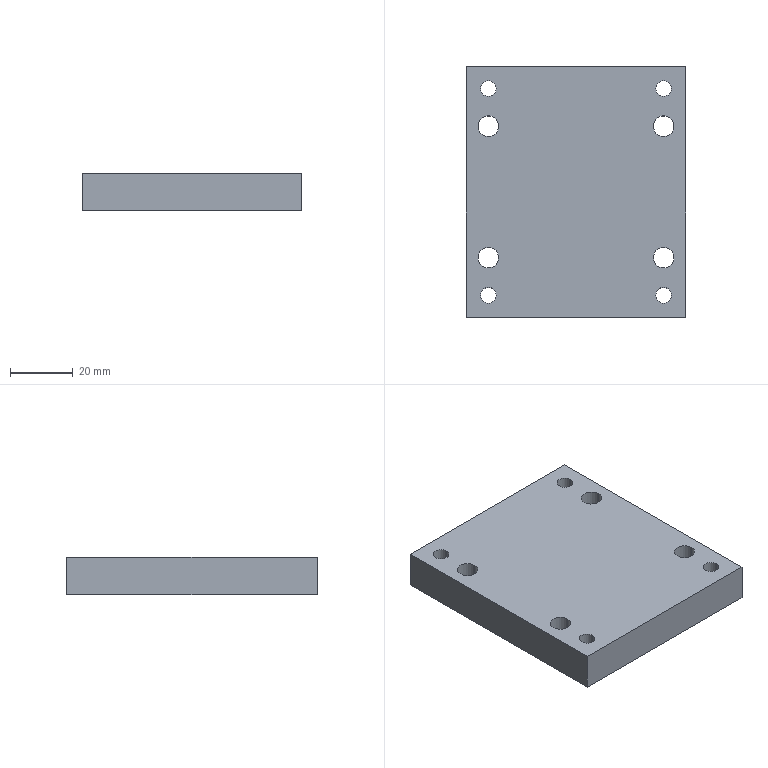Part | SolidWorks | features HoleWzd 2, Extrusion 1 | 1 solid | 34 faces | box 70 x 80 x 12 mm | volume 63058 mm3 | cylinder 24 | plane 10 | commonest cylinder face diameters 5 x8 6.6 x8 11 x8
STEP:
#1=CARTESIAN_POINT('',(33.5,-21.,6.4));
#2=VERTEX_POINT('',#1);
#3=CARTESIAN_POINT('',(22.5,-21.,6.4));
#4=VERTEX_POINT('',#3);
#5=CARTESIAN_POINT('',(28.,-21.,6.4));
#6=DIRECTION('',(0.,0.,-1.));
#7=DIRECTION('',(-1.,0.,0.));
#8=AXIS2_PLACEMENT_3D('',#5,#6,#7);
#9=CIRCLE('',#8,5.5);
#10=EDGE_CURVE('',#2,#4,#9,.T.);
#11=ORIENTED_EDGE('',*,*,#10,.F.);
#12=CARTESIAN_POINT('',(33.5,-21.,0.));
#13=VERTEX_POINT('',#12);
#14=CARTESIAN_POINT('',(33.5,-21.,0.));
#15=DIRECTION('',(0.,0.,-1.));
#16=VECTOR('',#15,1000.);
#17=LINE('',#14,#16);
#18=EDGE_CURVE('',#2,#13,#17,.T.);
#19=ORIENTED_EDGE('',*,*,#18,.T.);
#20=CARTESIAN_POINT('',(22.5,-21.,0.));
#21=VERTEX_POINT('',#20);
#22=CARTESIAN_POINT('',(28.,-21.,0.));
#23=DIRECTION('',(0.,0.,-1.));
#24=DIRECTION('',(-1.,0.,0.));
#25=AXIS2_PLACEMENT_3D('',#22,#23,#24);
#26=CIRCLE('',#25,5.5);
#27=EDGE_CURVE('',#13,#21,#26,.T.);
#28=ORIENTED_EDGE('',*,*,#27,.T.);
#29=CARTESIAN_POINT('',(22.5,-21.,0.));
#30=DIRECTION('',(0.,0.,-1.));
#31=VECTOR('',#30,1000.);
#32=LINE('',#29,#31);
#33=EDGE_CURVE('',#4,#21,#32,.T.);
#34=ORIENTED_EDGE('',*,*,#33,.F.);
#35=EDGE_LOOP('',(#11,#19,#28,#34));
#36=FACE_OUTER_BOUND('',#35,.T.);
#37=CARTESIAN_POINT('',(28.,-21.,0.));
#38=DIRECTION('',(0.,0.,-1.));
#39=DIRECTION('',(-1.,0.,0.));
#40=AXIS2_PLACEMENT_3D('',#37,#38,#39);
#41=CYLINDRICAL_SURFACE('',#40,5.5);
#42=ADVANCED_FACE('',(#36),#41,.F.);
#43=CARTESIAN_POINT('',(31.3,-21.,12.));
#44=VERTEX_POINT('',#43);
#45=CARTESIAN_POINT('',(24.7,-21.,12.));
#46=VERTEX_POINT('',#45);
#47=CARTESIAN_POINT('',(28.,-21.,12.));
#48=DIRECTION('',(0.,0.,-1.));
#49=DIRECTION('',(-1.,0.,0.));
#50=AXIS2_PLACEMENT_3D('',#47,#48,#49);
#51=CIRCLE('',#50,3.3);
#52=EDGE_CURVE('',#44,#46,#51,.T.);
#53=ORIENTED_EDGE('',*,*,#52,.F.);
#54=CARTESIAN_POINT('',(31.3,-21.,6.4));
#55=VERTEX_POINT('',#54);
#56=CARTESIAN_POINT('',(31.3,-21.,0.));
#57=DIRECTION('',(0.,0.,-1.));
#58=VECTOR('',#57,1000.);
#59=LINE('',#56,#58);
#60=EDGE_CURVE('',#44,#55,#59,.T.);
#61=ORIENTED_EDGE('',*,*,#60,.T.);
#62=CARTESIAN_POINT('',(24.7,-21.,6.4));
#63=VERTEX_POINT('',#62);
#64=CARTESIAN_POINT('',(28.,-21.,6.4));
#65=DIRECTION('',(0.,0.,-1.));
#66=DIRECTION('',(-1.,0.,0.));
#67=AXIS2_PLACEMENT_3D('',#64,#65,#66);
#68=CIRCLE('',#67,3.3);
#69=EDGE_CURVE('',#55,#63,#68,.T.);
#70=ORIENTED_EDGE('',*,*,#69,.T.);
#71=CARTESIAN_POINT('',(24.7,-21.,0.));
#72=DIRECTION('',(0.,0.,-1.));
#73=VECTOR('',#72,1000.);
#74=LINE('',#71,#73);
#75=EDGE_CURVE('',#46,#63,#74,.T.);
#76=ORIENTED_EDGE('',*,*,#75,.F.);
#77=EDGE_LOOP('',(#53,#61,#70,#76));
#78=FACE_OUTER_BOUND('',#77,.T.);
#79=CARTESIAN_POINT('',(28.,-21.,0.));
#80=DIRECTION('',(0.,0.,-1.));
#81=DIRECTION('',(-1.,0.,0.));
#82=AXIS2_PLACEMENT_3D('',#79,#80,#81);
#83=CYLINDRICAL_SURFACE('',#82,3.3);
#84=ADVANCED_FACE('',(#78),#83,.F.);
#85=CARTESIAN_POINT('',(33.5,21.,6.4));
#86=VERTEX_POINT('',#85);
#87=CARTESIAN_POINT('',(22.5,21.,6.4));
#88=VERTEX_POINT('',#87);
#89=CARTESIAN_POINT('',(28.,21.,6.4));
#90=DIRECTION('',(0.,0.,-1.));
#91=DIRECTION('',(-1.,0.,0.));
#92=AXIS2_PLACEMENT_3D('',#89,#90,#91);
#93=CIRCLE('',#92,5.5);
#94=EDGE_CURVE('',#86,#88,#93,.T.);
#95=ORIENTED_EDGE('',*,*,#94,.F.);
#96=CARTESIAN_POINT('',(33.5,21.,0.));
#97=VERTEX_POINT('',#96);
#98=CARTESIAN_POINT('',(33.5,21.,0.));
#99=DIRECTION('',(0.,0.,-1.));
#100=VECTOR('',#99,1000.);
#101=LINE('',#98,#100);
#102=EDGE_CURVE('',#86,#97,#101,.T.);
#103=ORIENTED_EDGE('',*,*,#102,.T.);
#104=CARTESIAN_POINT('',(22.5,21.,0.));
#105=VERTEX_POINT('',#104);
#106=CARTESIAN_POINT('',(28.,21.,0.));
#107=DIRECTION('',(0.,0.,-1.));
#108=DIRECTION('',(-1.,0.,0.));
#109=AXIS2_PLACEMENT_3D('',#106,#107,#108);
#110=CIRCLE('',#109,5.5);
#111=EDGE_CURVE('',#97,#105,#110,.T.);
#112=ORIENTED_EDGE('',*,*,#111,.T.);
#113=CARTESIAN_POINT('',(22.5,21.,0.));
#114=DIRECTION('',(0.,0.,-1.));
#115=VECTOR('',#114,1000.);
#116=LINE('',#113,#115);
#117=EDGE_CURVE('',#88,#105,#116,.T.);
#118=ORIENTED_EDGE('',*,*,#117,.F.);
#119=EDGE_LOOP('',(#95,#103,#112,#118));
#120=FACE_OUTER_BOUND('',#119,.T.);
#121=CARTESIAN_POINT('',(28.,21.,0.));
#122=DIRECTION('',(0.,0.,-1.));
#123=DIRECTION('',(-1.,0.,0.));
#124=AXIS2_PLACEMENT_3D('',#121,#122,#123);
#125=CYLINDRICAL_SURFACE('',#124,5.5);
#126=ADVANCED_FACE('',(#120),#125,.F.);
#127=CARTESIAN_POINT('',(31.3,21.,12.));
#128=VERTEX_POINT('',#127);
#129=CARTESIAN_POINT('',(24.7,21.,12.));
#130=VERTEX_POINT('',#129);
#131=CARTESIAN_POINT('',(28.,21.,12.));
#132=DIRECTION('',(0.,0.,-1.));
#133=DIRECTION('',(-1.,0.,0.));
#134=AXIS2_PLACEMENT_3D('',#131,#132,#133);
#135=CIRCLE('',#134,3.3);
#136=EDGE_CURVE('',#128,#130,#135,.T.);
#137=ORIENTED_EDGE('',*,*,#136,.F.);
#138=CARTESIAN_POINT('',(31.3,21.,6.4));
#139=VERTEX_POINT('',#138);
#140=CARTESIAN_POINT('',(31.3,21.,0.));
#141=DIRECTION('',(0.,0.,-1.));
#142=VECTOR('',#141,1000.);
#143=LINE('',#140,#142);
#144=EDGE_CURVE('',#128,#139,#143,.T.);
#145=ORIENTED_EDGE('',*,*,#144,.T.);
#146=CARTESIAN_POINT('',(24.7,21.,6.4));
#147=VERTEX_POINT('',#146);
#148=CARTESIAN_POINT('',(28.,21.,6.4));
#149=DIRECTION('',(0.,0.,-1.));
#150=DIRECTION('',(-1.,0.,0.));
#151=AXIS2_PLACEMENT_3D('',#148,#149,#150);
#152=CIRCLE('',#151,3.3);
#153=EDGE_CURVE('',#139,#147,#152,.T.);
#154=ORIENTED_EDGE('',*,*,#153,.T.);
#155=CARTESIAN_POINT('',(24.7,21.,0.));
#156=DIRECTION('',(0.,0.,-1.));
#157=VECTOR('',#156,1000.);
#158=LINE('',#155,#157);
#159=EDGE_CURVE('',#130,#147,#158,.T.);
#160=ORIENTED_EDGE('',*,*,#159,.F.);
#161=EDGE_LOOP('',(#137,#145,#154,#160));
#162=FACE_OUTER_BOUND('',#161,.T.);
#163=CARTESIAN_POINT('',(28.,21.,0.));
#164=DIRECTION('',(0.,0.,-1.));
#165=DIRECTION('',(-1.,0.,0.));
#166=AXIS2_PLACEMENT_3D('',#163,#164,#165);
#167=CYLINDRICAL_SURFACE('',#166,3.3);
#168=ADVANCED_FACE('',(#162),#167,.F.);
#169=CARTESIAN_POINT('',(-22.5,-21.,6.4));
#170=VERTEX_POINT('',#169);
#171=CARTESIAN_POINT('',(-33.5,-21.,6.4));
#172=VERTEX_POINT('',#171);
#173=CARTESIAN_POINT('',(-28.,-21.,6.4));
#174=DIRECTION('',(0.,0.,-1.));
#175=DIRECTION('',(-1.,0.,0.));
#176=AXIS2_PLACEMENT_3D('',#173,#174,#175);
#177=CIRCLE('',#176,5.5);
#178=EDGE_CURVE('',#170,#172,#177,.T.);
#179=ORIENTED_EDGE('',*,*,#178,.F.);
#180=CARTESIAN_POINT('',(-22.5,-21.,0.));
#181=VERTEX_POINT('',#180);
#182=CARTESIAN_POINT('',(-22.5,-21.,0.));
#183=DIRECTION('',(0.,0.,-1.));
#184=VECTOR('',#183,1000.);
#185=LINE('',#182,#184);
#186=EDGE_CURVE('',#170,#181,#185,.T.);
#187=ORIENTED_EDGE('',*,*,#186,.T.);
#188=CARTESIAN_POINT('',(-33.5,-21.,0.));
#189=VERTEX_POINT('',#188);
#190=CARTESIAN_POINT('',(-28.,-21.,0.));
#191=DIRECTION('',(0.,0.,-1.));
#192=DIRECTION('',(-1.,0.,0.));
#193=AXIS2_PLACEMENT_3D('',#190,#191,#192);
#194=CIRCLE('',#193,5.5);
#195=EDGE_CURVE('',#181,#189,#194,.T.);
#196=ORIENTED_EDGE('',*,*,#195,.T.);
#197=CARTESIAN_POINT('',(-33.5,-21.,0.));
#198=DIRECTION('',(0.,0.,-1.));
#199=VECTOR('',#198,1000.);
#200=LINE('',#197,#199);
#201=EDGE_CURVE('',#172,#189,#200,.T.);
#202=ORIENTED_EDGE('',*,*,#201,.F.);
#203=EDGE_LOOP('',(#179,#187,#196,#202));
#204=FACE_OUTER_BOUND('',#203,.T.);
#205=CARTESIAN_POINT('',(-28.,-21.,0.));
#206=DIRECTION('',(0.,0.,-1.));
#207=DIRECTION('',(-1.,0.,0.));
#208=AXIS2_PLACEMENT_3D('',#205,#206,#207);
#209=CYLINDRICAL_SURFACE('',#208,5.5);
#210=ADVANCED_FACE('',(#204),#209,.F.);
#211=CARTESIAN_POINT('',(-24.7,-21.,12.));
#212=VERTEX_POINT('',#211);
#213=CARTESIAN_POINT('',(-31.3,-21.,12.));
#214=VERTEX_POINT('',#213);
#215=CARTESIAN_POINT('',(-28.,-21.,12.));
#216=DIRECTION('',(0.,0.,-1.));
#217=DIRECTION('',(-1.,0.,0.));
#218=AXIS2_PLACEMENT_3D('',#215,#216,#217);
#219=CIRCLE('',#218,3.3);
#220=EDGE_CURVE('',#212,#214,#219,.T.);
#221=ORIENTED_EDGE('',*,*,#220,.F.);
#222=CARTESIAN_POINT('',(-24.7,-21.,6.4));
#223=VERTEX_POINT('',#222);
#224=CARTESIAN_POINT('',(-24.7,-21.,0.));
#225=DIRECTION('',(0.,0.,-1.));
#226=VECTOR('',#225,1000.);
#227=LINE('',#224,#226);
#228=EDGE_CURVE('',#212,#223,#227,.T.);
#229=ORIENTED_EDGE('',*,*,#228,.T.);
#230=CARTESIAN_POINT('',(-31.3,-21.,6.4));
#231=VERTEX_POINT('',#230);
#232=CARTESIAN_POINT('',(-28.,-21.,6.4));
#233=DIRECTION('',(0.,0.,-1.));
#234=DIRECTION('',(-1.,0.,0.));
#235=AXIS2_PLACEMENT_3D('',#232,#233,#234);
#236=CIRCLE('',#235,3.3);
#237=EDGE_CURVE('',#223,#231,#236,.T.);
#238=ORIENTED_EDGE('',*,*,#237,.T.);
#239=CARTESIAN_POINT('',(-31.3,-21.,0.));
#240=DIRECTION('',(0.,0.,-1.));
#241=VECTOR('',#240,1000.);
#242=LINE('',#239,#241);
#243=EDGE_CURVE('',#214,#231,#242,.T.);
#244=ORIENTED_EDGE('',*,*,#243,.F.);
#245=EDGE_LOOP('',(#221,#229,#238,#244));
#246=FACE_OUTER_BOUND('',#245,.T.);
#247=CARTESIAN_POINT('',(-28.,-21.,0.));
#248=DIRECTION('',(0.,0.,-1.));
#249=DIRECTION('',(-1.,0.,0.));
#250=AXIS2_PLACEMENT_3D('',#247,#248,#249);
#251=CYLINDRICAL_SURFACE('',#250,3.3);
#252=ADVANCED_FACE('',(#246),#251,.F.);
#253=CARTESIAN_POINT('',(-22.5,21.,6.4));
#254=VERTEX_POINT('',#253);
#255=CARTESIAN_POINT('',(-33.5,21.,6.4));
#256=VERTEX_POINT('',#255);
#257=CARTESIAN_POINT('',(-28.,21.,6.4));
#258=DIRECTION('',(0.,0.,-1.));
#259=DIRECTION('',(-1.,0.,0.));
#260=AXIS2_PLACEMENT_3D('',#257,#258,#259);
#261=CIRCLE('',#260,5.5);
#262=EDGE_CURVE('',#254,#256,#261,.T.);
#263=ORIENTED_EDGE('',*,*,#262,.F.);
#264=CARTESIAN_POINT('',(-22.5,21.,0.));
#265=VERTEX_POINT('',#264);
#266=CARTESIAN_POINT('',(-22.5,21.,0.));
#267=DIRECTION('',(0.,0.,-1.));
#268=VECTOR('',#267,1000.);
#269=LINE('',#266,#268);
#270=EDGE_CURVE('',#254,#265,#269,.T.);
#271=ORIENTED_EDGE('',*,*,#270,.T.);
#272=CARTESIAN_POINT('',(-33.5,21.,0.));
#273=VERTEX_POINT('',#272);
#274=CARTESIAN_POINT('',(-28.,21.,0.));
#275=DIRECTION('',(0.,0.,-1.));
#276=DIRECTION('',(-1.,0.,0.));
#277=AXIS2_PLACEMENT_3D('',#274,#275,#276);
#278=CIRCLE('',#277,5.5);
#279=EDGE_CURVE('',#265,#273,#278,.T.);
#280=ORIENTED_EDGE('',*,*,#279,.T.);
#281=CARTESIAN_POINT('',(-33.5,21.,0.));
#282=DIRECTION('',(0.,0.,-1.));
#283=VECTOR('',#282,1000.);
#284=LINE('',#281,#283);
#285=EDGE_CURVE('',#256,#273,#284,.T.);
#286=ORIENTED_EDGE('',*,*,#285,.F.);
#287=EDGE_LOOP('',(#263,#271,#280,#286));
#288=FACE_OUTER_BOUND('',#287,.T.);
#289=CARTESIAN_POINT('',(-28.,21.,0.));
#290=DIRECTION('',(0.,0.,-1.));
#291=DIRECTION('',(-1.,0.,0.));
#292=AXIS2_PLACEMENT_3D('',#289,#290,#291);
#293=CYLINDRICAL_SURFACE('',#292,5.5);
#294=ADVANCED_FACE('',(#288),#293,.F.);
#295=CARTESIAN_POINT('',(-24.7,21.,12.));
#296=VERTEX_POINT('',#295);
#297=CARTESIAN_POINT('',(-31.3,21.,12.));
#298=VERTEX_POINT('',#297);
#299=CARTESIAN_POINT('',(-28.,21.,12.));
#300=DIRECTION('',(0.,0.,-1.));
#301=DIRECTION('',(-1.,0.,0.));
#302=AXIS2_PLACEMENT_3D('',#299,#300,#301);
#303=CIRCLE('',#302,3.3);
#304=EDGE_CURVE('',#296,#298,#303,.T.);
#305=ORIENTED_EDGE('',*,*,#304,.F.);
#306=CARTESIAN_POINT('',(-24.7,21.,6.4));
#307=VERTEX_POINT('',#306);
#308=CARTESIAN_POINT('',(-24.7,21.,0.));
#309=DIRECTION('',(0.,0.,-1.));
#310=VECTOR('',#309,1000.);
#311=LINE('',#308,#310);
#312=EDGE_CURVE('',#296,#307,#311,.T.);
#313=ORIENTED_EDGE('',*,*,#312,.T.);
#314=CARTESIAN_POINT('',(-31.3,21.,6.4));
#315=VERTEX_POINT('',#314);
#316=CARTESIAN_POINT('',(-28.,21.,6.4));
#317=DIRECTION('',(0.,0.,-1.));
#318=DIRECTION('',(-1.,0.,0.));
#319=AXIS2_PLACEMENT_3D('',#316,#317,#318);
#320=CIRCLE('',#319,3.3);
#321=EDGE_CURVE('',#307,#315,#320,.T.);
#322=ORIENTED_EDGE('',*,*,#321,.T.);
#323=CARTESIAN_POINT('',(-31.3,21.,0.));
#324=DIRECTION('',(0.,0.,-1.));
#325=VECTOR('',#324,1000.);
#326=LINE('',#323,#325);
#327=EDGE_CURVE('',#298,#315,#326,.T.);
#328=ORIENTED_EDGE('',*,*,#327,.F.);
#329=EDGE_LOOP('',(#305,#313,#322,#328));
#330=FACE_OUTER_BOUND('',#329,.T.);
#331=CARTESIAN_POINT('',(-28.,21.,0.));
#332=DIRECTION('',(0.,0.,-1.));
#333=DIRECTION('',(-1.,0.,0.));
#334=AXIS2_PLACEMENT_3D('',#331,#332,#333);
#335=CYLINDRICAL_SURFACE('',#334,3.3);
#336=ADVANCED_FACE('',(#330),#335,.F.);
#337=CARTESIAN_POINT('',(-25.5,33.,12.));
#338=VERTEX_POINT('',#337);
#339=CARTESIAN_POINT('',(-30.5,33.,12.));
#340=VERTEX_POINT('',#339);
#341=CARTESIAN_POINT('',(-28.,33.,12.));
#342=DIRECTION('',(0.,0.,-1.));
#343=DIRECTION('',(-1.,0.,0.));
#344=AXIS2_PLACEMENT_3D('',#341,#342,#343);
#345=CIRCLE('',#344,2.5);
#346=EDGE_CURVE('',#338,#340,#345,.T.);
#347=ORIENTED_EDGE('',*,*,#346,.F.);
#348=CARTESIAN_POINT('',(-25.5,33.,0.));
#349=VERTEX_POINT('',#348);
#350=CARTESIAN_POINT('',(-25.5,33.,0.));
#351=DIRECTION('',(0.,0.,-1.));
#352=VECTOR('',#351,1000.);
#353=LINE('',#350,#352);
#354=EDGE_CURVE('',#338,#349,#353,.T.);
#355=ORIENTED_EDGE('',*,*,#354,.T.);
#356=CARTESIAN_POINT('',(-30.5,33.,0.));
#357=VERTEX_POINT('',#356);
#358=CARTESIAN_POINT('',(-28.,33.,0.));
#359=DIRECTION('',(0.,0.,-1.));
#360=DIRECTION('',(-1.,0.,0.));
#361=AXIS2_PLACEMENT_3D('',#358,#359,#360);
#362=CIRCLE('',#361,2.5);
#363=EDGE_CURVE('',#349,#357,#362,.T.);
#364=ORIENTED_EDGE('',*,*,#363,.T.);
#365=CARTESIAN_POINT('',(-30.5,33.,0.));
#366=DIRECTION('',(0.,0.,-1.));
#367=VECTOR('',#366,1000.);
#368=LINE('',#365,#367);
#369=EDGE_CURVE('',#340,#357,#368,.T.);
#370=ORIENTED_EDGE('',*,*,#369,.F.);
#371=EDGE_LOOP('',(#347,#355,#364,#370));
#372=FACE_OUTER_BOUND('',#371,.T.);
#373=CARTESIAN_POINT('',(-28.,33.,0.));
#374=DIRECTION('',(0.,0.,-1.));
#375=DIRECTION('',(-1.,0.,0.));
#376=AXIS2_PLACEMENT_3D('',#373,#374,#375);
#377=CYLINDRICAL_SURFACE('',#376,2.5);
#378=ADVANCED_FACE('',(#372),#377,.F.);
#379=CARTESIAN_POINT('',(-25.5,-33.,12.));
#380=VERTEX_POINT('',#379);
#381=CARTESIAN_POINT('',(-30.5,-33.,12.));
#382=VERTEX_POINT('',#381);
#383=CARTESIAN_POINT('',(-28.,-33.,12.));
#384=DIRECTION('',(0.,0.,-1.));
#385=DIRECTION('',(-1.,0.,0.));
#386=AXIS2_PLACEMENT_3D('',#383,#384,#385);
#387=CIRCLE('',#386,2.5);
#388=EDGE_CURVE('',#380,#382,#387,.T.);
#389=ORIENTED_EDGE('',*,*,#388,.F.);
#390=CARTESIAN_POINT('',(-25.5,-33.,0.));
#391=VERTEX_POINT('',#390);
#392=CARTESIAN_POINT('',(-25.5,-33.,0.));
#393=DIRECTION('',(0.,0.,-1.));
#394=VECTOR('',#393,1000.);
#395=LINE('',#392,#394);
#396=EDGE_CURVE('',#380,#391,#395,.T.);
#397=ORIENTED_EDGE('',*,*,#396,.T.);
#398=CARTESIAN_POINT('',(-30.5,-33.,0.));
#399=VERTEX_POINT('',#398);
#400=CARTESIAN_POINT('',(-28.,-33.,0.));
#401=DIRECTION('',(0.,0.,-1.));
#402=DIRECTION('',(-1.,0.,0.));
#403=AXIS2_PLACEMENT_3D('',#400,#401,#402);
#404=CIRCLE('',#403,2.5);
#405=EDGE_CURVE('',#391,#399,#404,.T.);
#406=ORIENTED_EDGE('',*,*,#405,.T.);
#407=CARTESIAN_POINT('',(-30.5,-33.,0.));
#408=DIRECTION('',(0.,0.,-1.));
#409=VECTOR('',#408,1000.);
#410=LINE('',#407,#409);
#411=EDGE_CURVE('',#382,#399,#410,.T.);
#412=ORIENTED_EDGE('',*,*,#411,.F.);
#413=EDGE_LOOP('',(#389,#397,#406,#412));
#414=FACE_OUTER_BOUND('',#413,.T.);
#415=CARTESIAN_POINT('',(-28.,-33.,0.));
#416=DIRECTION('',(0.,0.,-1.));
#417=DIRECTION('',(-1.,0.,0.));
#418=AXIS2_PLACEMENT_3D('',#415,#416,#417);
#419=CYLINDRICAL_SURFACE('',#418,2.5);
#420=ADVANCED_FACE('',(#414),#419,.F.);
#421=CARTESIAN_POINT('',(30.5,-33.,12.));
#422=VERTEX_POINT('',#421);
#423=CARTESIAN_POINT('',(25.5,-33.,12.));
#424=VERTEX_POINT('',#423);
#425=CARTESIAN_POINT('',(28.,-33.,12.));
#426=DIRECTION('',(0.,0.,-1.));
#427=DIRECTION('',(-1.,0.,0.));
#428=AXIS2_PLACEMENT_3D('',#425,#426,#427);
#429=CIRCLE('',#428,2.5);
#430=EDGE_CURVE('',#422,#424,#429,.T.);
#431=ORIENTED_EDGE('',*,*,#430,.F.);
#432=CARTESIAN_POINT('',(30.5,-33.,0.));
#433=VERTEX_POINT('',#432);
#434=CARTESIAN_POINT('',(30.5,-33.,0.));
#435=DIRECTION('',(0.,0.,-1.));
#436=VECTOR('',#435,1000.);
#437=LINE('',#434,#436);
#438=EDGE_CURVE('',#422,#433,#437,.T.);
#439=ORIENTED_EDGE('',*,*,#438,.T.);
#440=CARTESIAN_POINT('',(25.5,-33.,0.));
#441=VERTEX_POINT('',#440);
#442=CARTESIAN_POINT('',(28.,-33.,0.));
#443=DIRECTION('',(0.,0.,-1.));
#444=DIRECTION('',(-1.,0.,0.));
#445=AXIS2_PLACEMENT_3D('',#442,#443,#444);
#446=CIRCLE('',#445,2.5);
#447=EDGE_CURVE('',#433,#441,#446,.T.);
#448=ORIENTED_EDGE('',*,*,#447,.T.);
#449=CARTESIAN_POINT('',(25.5,-33.,0.));
#450=DIRECTION('',(0.,0.,-1.));
#451=VECTOR('',#450,1000.);
#452=LINE('',#449,#451);
#453=EDGE_CURVE('',#424,#441,#452,.T.);
#454=ORIENTED_EDGE('',*,*,#453,.F.);
#455=EDGE_LOOP('',(#431,#439,#448,#454));
#456=FACE_OUTER_BOUND('',#455,.T.);
#457=CARTESIAN_POINT('',(28.,-33.,0.));
#458=DIRECTION('',(0.,0.,-1.));
#459=DIRECTION('',(-1.,0.,0.));
#460=AXIS2_PLACEMENT_3D('',#457,#458,#459);
#461=CYLINDRICAL_SURFACE('',#460,2.5);
#462=ADVANCED_FACE('',(#456),#461,.F.);
#463=CARTESIAN_POINT('',(30.5,33.,12.));
#464=VERTEX_POINT('',#463);
#465=CARTESIAN_POINT('',(25.5,33.,12.));
#466=VERTEX_POINT('',#465);
#467=CARTESIAN_POINT('',(28.,33.,12.));
#468=DIRECTION('',(0.,0.,-1.));
#469=DIRECTION('',(-1.,0.,0.));
#470=AXIS2_PLACEMENT_3D('',#467,#468,#469);
#471=CIRCLE('',#470,2.5);
#472=EDGE_CURVE('',#464,#466,#471,.T.);
#473=ORIENTED_EDGE('',*,*,#472,.F.);
#474=CARTESIAN_POINT('',(30.5,33.,0.));
#475=VERTEX_POINT('',#474);
#476=CARTESIAN_POINT('',(30.5,33.,0.));
#477=DIRECTION('',(0.,0.,-1.));
#478=VECTOR('',#477,1000.);
#479=LINE('',#476,#478);
#480=EDGE_CURVE('',#464,#475,#479,.T.);
#481=ORIENTED_EDGE('',*,*,#480,.T.);
#482=CARTESIAN_POINT('',(25.5,33.,0.));
#483=VERTEX_POINT('',#482);
#484=CARTESIAN_POINT('',(28.,33.,0.));
#485=DIRECTION('',(0.,0.,-1.));
#486=DIRECTION('',(-1.,0.,0.));
#487=AXIS2_PLACEMENT_3D('',#484,#485,#486);
#488=CIRCLE('',#487,2.5);
#489=EDGE_CURVE('',#475,#483,#488,.T.);
#490=ORIENTED_EDGE('',*,*,#489,.T.);
#491=CARTESIAN_POINT('',(25.5,33.,0.));
#492=DIRECTION('',(0.,0.,-1.));
#493=VECTOR('',#492,1000.);
#494=LINE('',#491,#493);
#495=EDGE_CURVE('',#466,#483,#494,.T.);
#496=ORIENTED_EDGE('',*,*,#495,.F.);
#497=EDGE_LOOP('',(#473,#481,#490,#496));
#498=FACE_OUTER_BOUND('',#497,.T.);
#499=CARTESIAN_POINT('',(28.,33.,0.));
#500=DIRECTION('',(0.,0.,-1.));
#501=DIRECTION('',(-1.,0.,0.));
#502=AXIS2_PLACEMENT_3D('',#499,#500,#501);
#503=CYLINDRICAL_SURFACE('',#502,2.5);
#504=ADVANCED_FACE('',(#498),#503,.F.);
#505=CARTESIAN_POINT('',(35.,-40.,0.));
#506=VERTEX_POINT('',#505);
#507=CARTESIAN_POINT('',(35.,40.,0.));
#508=VERTEX_POINT('',#507);
#509=CARTESIAN_POINT('',(35.,40.,0.));
#510=DIRECTION('',(0.,1.,0.));
#511=VECTOR('',#510,1000.);
#512=LINE('',#509,#511);
#513=EDGE_CURVE('',#506,#508,#512,.T.);
#514=ORIENTED_EDGE('',*,*,#513,.T.);
#515=CARTESIAN_POINT('',(35.,40.,12.));
#516=VERTEX_POINT('',#515);
#517=CARTESIAN_POINT('',(35.,40.,12.));
#518=DIRECTION('',(0.,0.,-1.));
#519=VECTOR('',#518,1000.);
#520=LINE('',#517,#519);
#521=EDGE_CURVE('',#516,#508,#520,.T.);
#522=ORIENTED_EDGE('',*,*,#521,.F.);
#523=CARTESIAN_POINT('',(35.,-40.,12.));
#524=VERTEX_POINT('',#523);
#525=CARTESIAN_POINT('',(35.,40.,12.));
#526=DIRECTION('',(0.,1.,0.));
#527=VECTOR('',#526,1000.);
#528=LINE('',#525,#527);
#529=EDGE_CURVE('',#524,#516,#528,.T.);
#530=ORIENTED_EDGE('',*,*,#529,.F.);
#531=CARTESIAN_POINT('',(35.,-40.,12.));
#532=DIRECTION('',(0.,0.,-1.));
#533=VECTOR('',#532,1000.);
#534=LINE('',#531,#533);
#535=EDGE_CURVE('',#524,#506,#534,.T.);
#536=ORIENTED_EDGE('',*,*,#535,.T.);
#537=EDGE_LOOP('',(#514,#522,#530,#536));
#538=FACE_OUTER_BOUND('',#537,.T.);
#539=CARTESIAN_POINT('',(35.,40.,12.));
#540=DIRECTION('',(-1.,0.,0.));
#541=DIRECTION('',(0.,-1.,0.));
#542=AXIS2_PLACEMENT_3D('',#539,#540,#541);
#543=PLANE('',#542);
#544=ADVANCED_FACE('',(#538),#543,.F.);
#545=CARTESIAN_POINT('',(-35.,40.,0.));
#546=VERTEX_POINT('',#545);
#547=CARTESIAN_POINT('',(-35.,40.,0.));
#548=DIRECTION('',(-1.,0.,0.));
#549=VECTOR('',#548,1000.);
#550=LINE('',#547,#549);
#551=EDGE_CURVE('',#508,#546,#550,.T.);
#552=ORIENTED_EDGE('',*,*,#551,.T.);
#553=CARTESIAN_POINT('',(-35.,40.,12.));
#554=VERTEX_POINT('',#553);
#555=CARTESIAN_POINT('',(-35.,40.,12.));
#556=DIRECTION('',(0.,0.,-1.));
#557=VECTOR('',#556,1000.);
#558=LINE('',#555,#557);
#559=EDGE_CURVE('',#554,#546,#558,.T.);
#560=ORIENTED_EDGE('',*,*,#559,.F.);
#561=CARTESIAN_POINT('',(-35.,40.,12.));
#562=DIRECTION('',(-1.,0.,0.));
#563=VECTOR('',#562,1000.);
#564=LINE('',#561,#563);
#565=EDGE_CURVE('',#516,#554,#564,.T.);
#566=ORIENTED_EDGE('',*,*,#565,.F.);
#567=ORIENTED_EDGE('',*,*,#521,.T.);
#568=EDGE_LOOP('',(#552,#560,#566,#567));
#569=FACE_OUTER_BOUND('',#568,.T.);
#570=CARTESIAN_POINT('',(-35.,40.,12.));
#571=DIRECTION('',(0.,-1.,0.));
#572=DIRECTION('',(0.,0.,-1.));
#573=AXIS2_PLACEMENT_3D('',#570,#571,#572);
#574=PLANE('',#573);
#575=ADVANCED_FACE('',(#569),#574,.F.);
#576=CARTESIAN_POINT('',(-35.,-40.,0.));
#577=VERTEX_POINT('',#576);
#578=CARTESIAN_POINT('',(-35.,40.,0.));
#579=DIRECTION('',(0.,-1.,0.));
#580=VECTOR('',#579,1000.);
#581=LINE('',#578,#580);
#582=EDGE_CURVE('',#546,#577,#581,.T.);
#583=ORIENTED_EDGE('',*,*,#582,.T.);
#584=CARTESIAN_POINT('',(-35.,-40.,12.));
#585=VERTEX_POINT('',#584);
#586=CARTESIAN_POINT('',(-35.,-40.,12.));
#587=DIRECTION('',(0.,0.,-1.));
#588=VECTOR('',#587,1000.);
#589=LINE('',#586,#588);
#590=EDGE_CURVE('',#585,#577,#589,.T.);
#591=ORIENTED_EDGE('',*,*,#590,.F.);
#592=CARTESIAN_POINT('',(-35.,40.,12.));
#593=DIRECTION('',(0.,-1.,0.));
#594=VECTOR('',#593,1000.);
#595=LINE('',#592,#594);
#596=EDGE_CURVE('',#554,#585,#595,.T.);
#597=ORIENTED_EDGE('',*,*,#596,.F.);
#598=ORIENTED_EDGE('',*,*,#559,.T.);
#599=EDGE_LOOP('',(#583,#591,#597,#598));
#600=FACE_OUTER_BOUND('',#599,.T.);
#601=CARTESIAN_POINT('',(-35.,40.,12.));
#602=DIRECTION('',(1.,0.,0.));
#603=DIRECTION('',(0.,0.,-1.));
#604=AXIS2_PLACEMENT_3D('',#601,#602,#603);
#605=PLANE('',#604);
#606=ADVANCED_FACE('',(#600),#605,.F.);
#607=CARTESIAN_POINT('',(-35.,-40.,0.));
#608=DIRECTION('',(1.,0.,0.));
#609=VECTOR('',#608,1000.);
#610=LINE('',#607,#609);
#611=EDGE_CURVE('',#577,#506,#610,.T.);
#612=ORIENTED_EDGE('',*,*,#611,.T.);
#613=ORIENTED_EDGE('',*,*,#535,.F.);
#614=CARTESIAN_POINT('',(-35.,-40.,12.));
#615=DIRECTION('',(1.,0.,0.));
#616=VECTOR('',#615,1000.);
#617=LINE('',#614,#616);
#618=EDGE_CURVE('',#585,#524,#617,.T.);
#619=ORIENTED_EDGE('',*,*,#618,.F.);
#620=ORIENTED_EDGE('',*,*,#590,.T.);
#621=EDGE_LOOP('',(#612,#613,#619,#620));
#622=FACE_OUTER_BOUND('',#621,.T.);
#623=CARTESIAN_POINT('',(-35.,-40.,12.));
#624=DIRECTION('',(0.,1.,0.));
#625=DIRECTION('',(0.,0.,1.));
#626=AXIS2_PLACEMENT_3D('',#623,#624,#625);
#627=PLANE('',#626);
#628=ADVANCED_FACE('',(#622),#627,.F.);
#629=CARTESIAN_POINT('',(28.,-21.,12.));
#630=DIRECTION('',(0.,0.,-1.));
#631=DIRECTION('',(-1.,0.,0.));
#632=AXIS2_PLACEMENT_3D('',#629,#630,#631);
#633=CIRCLE('',#632,3.3);
#634=EDGE_CURVE('',#46,#44,#633,.T.);
#635=ORIENTED_EDGE('',*,*,#634,.T.);
#636=ORIENTED_EDGE('',*,*,#52,.T.);
#637=EDGE_LOOP('',(#635,#636));
#638=FACE_BOUND('',#637,.T.);
#639=CARTESIAN_POINT('',(28.,21.,12.));
#640=DIRECTION('',(0.,0.,-1.));
#641=DIRECTION('',(-1.,0.,0.));
#642=AXIS2_PLACEMENT_3D('',#639,#640,#641);
#643=CIRCLE('',#642,3.3);
#644=EDGE_CURVE('',#130,#128,#643,.T.);
#645=ORIENTED_EDGE('',*,*,#644,.T.);
#646=ORIENTED_EDGE('',*,*,#136,.T.);
#647=EDGE_LOOP('',(#645,#646));
#648=FACE_BOUND('',#647,.T.);
#649=CARTESIAN_POINT('',(-28.,-21.,12.));
#650=DIRECTION('',(0.,0.,-1.));
#651=DIRECTION('',(-1.,0.,0.));
#652=AXIS2_PLACEMENT_3D('',#649,#650,#651);
#653=CIRCLE('',#652,3.3);
#654=EDGE_CURVE('',#214,#212,#653,.T.);
#655=ORIENTED_EDGE('',*,*,#654,.T.);
#656=ORIENTED_EDGE('',*,*,#220,.T.);
#657=EDGE_LOOP('',(#655,#656));
#658=FACE_BOUND('',#657,.T.);
#659=CARTESIAN_POINT('',(-28.,21.,12.));
#660=DIRECTION('',(0.,0.,-1.));
#661=DIRECTION('',(-1.,0.,0.));
#662=AXIS2_PLACEMENT_3D('',#659,#660,#661);
#663=CIRCLE('',#662,3.3);
#664=EDGE_CURVE('',#298,#296,#663,.T.);
#665=ORIENTED_EDGE('',*,*,#664,.T.);
#666=ORIENTED_EDGE('',*,*,#304,.T.);
#667=EDGE_LOOP('',(#665,#666));
#668=FACE_BOUND('',#667,.T.);
#669=CARTESIAN_POINT('',(-28.,33.,12.));
#670=DIRECTION('',(0.,0.,-1.));
#671=DIRECTION('',(-1.,0.,0.));
#672=AXIS2_PLACEMENT_3D('',#669,#670,#671);
#673=CIRCLE('',#672,2.5);
#674=EDGE_CURVE('',#340,#338,#673,.T.);
#675=ORIENTED_EDGE('',*,*,#674,.T.);
#676=ORIENTED_EDGE('',*,*,#346,.T.);
#677=EDGE_LOOP('',(#675,#676));
#678=FACE_BOUND('',#677,.T.);
#679=CARTESIAN_POINT('',(-28.,-33.,12.));
#680=DIRECTION('',(0.,0.,-1.));
#681=DIRECTION('',(-1.,0.,0.));
#682=AXIS2_PLACEMENT_3D('',#679,#680,#681);
#683=CIRCLE('',#682,2.5);
#684=EDGE_CURVE('',#382,#380,#683,.T.);
#685=ORIENTED_EDGE('',*,*,#684,.T.);
#686=ORIENTED_EDGE('',*,*,#388,.T.);
#687=EDGE_LOOP('',(#685,#686));
#688=FACE_BOUND('',#687,.T.);
#689=CARTESIAN_POINT('',(28.,-33.,12.));
#690=DIRECTION('',(0.,0.,-1.));
#691=DIRECTION('',(-1.,0.,0.));
#692=AXIS2_PLACEMENT_3D('',#689,#690,#691);
#693=CIRCLE('',#692,2.5);
#694=EDGE_CURVE('',#424,#422,#693,.T.);
#695=ORIENTED_EDGE('',*,*,#694,.T.);
#696=ORIENTED_EDGE('',*,*,#430,.T.);
#697=EDGE_LOOP('',(#695,#696));
#698=FACE_BOUND('',#697,.T.);
#699=CARTESIAN_POINT('',(28.,33.,12.));
#700=DIRECTION('',(0.,0.,-1.));
#701=DIRECTION('',(-1.,0.,0.));
#702=AXIS2_PLACEMENT_3D('',#699,#700,#701);
#703=CIRCLE('',#702,2.5);
#704=EDGE_CURVE('',#466,#464,#703,.T.);
#705=ORIENTED_EDGE('',*,*,#704,.T.);
#706=ORIENTED_EDGE('',*,*,#472,.T.);
#707=EDGE_LOOP('',(#705,#706));
#708=FACE_BOUND('',#707,.T.);
#709=ORIENTED_EDGE('',*,*,#529,.T.);
#710=ORIENTED_EDGE('',*,*,#565,.T.);
#711=ORIENTED_EDGE('',*,*,#596,.T.);
#712=ORIENTED_EDGE('',*,*,#618,.T.);
#713=EDGE_LOOP('',(#709,#710,#711,#712));
#714=FACE_OUTER_BOUND('',#713,.T.);
#715=CARTESIAN_POINT('',(0.,0.,12.));
#716=DIRECTION('',(0.,0.,1.));
#717=DIRECTION('',(1.,0.,0.));
#718=AXIS2_PLACEMENT_3D('',#715,#716,#717);
#719=PLANE('',#718);
#720=ADVANCED_FACE('',(#638,#648,#658,#668,#678,#688,#698,#708,#714),#719,.T.);
#721=CARTESIAN_POINT('',(28.,-21.,0.));
#722=DIRECTION('',(0.,0.,-1.));
#723=DIRECTION('',(-1.,0.,0.));
#724=AXIS2_PLACEMENT_3D('',#721,#722,#723);
#725=CIRCLE('',#724,5.5);
#726=EDGE_CURVE('',#21,#13,#725,.T.);
#727=ORIENTED_EDGE('',*,*,#726,.F.);
#728=ORIENTED_EDGE('',*,*,#27,.F.);
#729=EDGE_LOOP('',(#727,#728));
#730=FACE_BOUND('',#729,.T.);
#731=CARTESIAN_POINT('',(28.,21.,0.));
#732=DIRECTION('',(0.,0.,-1.));
#733=DIRECTION('',(-1.,0.,0.));
#734=AXIS2_PLACEMENT_3D('',#731,#732,#733);
#735=CIRCLE('',#734,5.5);
#736=EDGE_CURVE('',#105,#97,#735,.T.);
#737=ORIENTED_EDGE('',*,*,#736,.F.);
#738=ORIENTED_EDGE('',*,*,#111,.F.);
#739=EDGE_LOOP('',(#737,#738));
#740=FACE_BOUND('',#739,.T.);
#741=CARTESIAN_POINT('',(-28.,-21.,0.));
#742=DIRECTION('',(0.,0.,-1.));
#743=DIRECTION('',(-1.,0.,0.));
#744=AXIS2_PLACEMENT_3D('',#741,#742,#743);
#745=CIRCLE('',#744,5.5);
#746=EDGE_CURVE('',#189,#181,#745,.T.);
#747=ORIENTED_EDGE('',*,*,#746,.F.);
#748=ORIENTED_EDGE('',*,*,#195,.F.);
#749=EDGE_LOOP('',(#747,#748));
#750=FACE_BOUND('',#749,.T.);
#751=CARTESIAN_POINT('',(-28.,21.,0.));
#752=DIRECTION('',(0.,0.,-1.));
#753=DIRECTION('',(-1.,0.,0.));
#754=AXIS2_PLACEMENT_3D('',#751,#752,#753);
#755=CIRCLE('',#754,5.5);
#756=EDGE_CURVE('',#273,#265,#755,.T.);
#757=ORIENTED_EDGE('',*,*,#756,.F.);
#758=ORIENTED_EDGE('',*,*,#279,.F.);
#759=EDGE_LOOP('',(#757,#758));
#760=FACE_BOUND('',#759,.T.);
#761=CARTESIAN_POINT('',(-28.,33.,0.));
#762=DIRECTION('',(0.,0.,-1.));
#763=DIRECTION('',(-1.,0.,0.));
#764=AXIS2_PLACEMENT_3D('',#761,#762,#763);
#765=CIRCLE('',#764,2.5);
#766=EDGE_CURVE('',#357,#349,#765,.T.);
#767=ORIENTED_EDGE('',*,*,#766,.F.);
#768=ORIENTED_EDGE('',*,*,#363,.F.);
#769=EDGE_LOOP('',(#767,#768));
#770=FACE_BOUND('',#769,.T.);
#771=CARTESIAN_POINT('',(-28.,-33.,0.));
#772=DIRECTION('',(0.,0.,-1.));
#773=DIRECTION('',(-1.,0.,0.));
#774=AXIS2_PLACEMENT_3D('',#771,#772,#773);
#775=CIRCLE('',#774,2.5);
#776=EDGE_CURVE('',#399,#391,#775,.T.);
#777=ORIENTED_EDGE('',*,*,#776,.F.);
#778=ORIENTED_EDGE('',*,*,#405,.F.);
#779=EDGE_LOOP('',(#777,#778));
#780=FACE_BOUND('',#779,.T.);
#781=CARTESIAN_POINT('',(28.,-33.,0.));
#782=DIRECTION('',(0.,0.,-1.));
#783=DIRECTION('',(-1.,0.,0.));
#784=AXIS2_PLACEMENT_3D('',#781,#782,#783);
#785=CIRCLE('',#784,2.5);
#786=EDGE_CURVE('',#441,#433,#785,.T.);
#787=ORIENTED_EDGE('',*,*,#786,.F.);
#788=ORIENTED_EDGE('',*,*,#447,.F.);
#789=EDGE_LOOP('',(#787,#788));
#790=FACE_BOUND('',#789,.T.);
#791=CARTESIAN_POINT('',(28.,33.,0.));
#792=DIRECTION('',(0.,0.,-1.));
#793=DIRECTION('',(-1.,0.,0.));
#794=AXIS2_PLACEMENT_3D('',#791,#792,#793);
#795=CIRCLE('',#794,2.5);
#796=EDGE_CURVE('',#483,#475,#795,.T.);
#797=ORIENTED_EDGE('',*,*,#796,.F.);
#798=ORIENTED_EDGE('',*,*,#489,.F.);
#799=EDGE_LOOP('',(#797,#798));
#800=FACE_BOUND('',#799,.T.);
#801=ORIENTED_EDGE('',*,*,#513,.F.);
#802=ORIENTED_EDGE('',*,*,#611,.F.);
#803=ORIENTED_EDGE('',*,*,#582,.F.);
#804=ORIENTED_EDGE('',*,*,#551,.F.);
#805=EDGE_LOOP('',(#801,#802,#803,#804));
#806=FACE_OUTER_BOUND('',#805,.T.);
#807=CARTESIAN_POINT('',(0.,0.,0.));
#808=DIRECTION('',(0.,0.,1.));
#809=DIRECTION('',(1.,0.,0.));
#810=AXIS2_PLACEMENT_3D('',#807,#808,#809);
#811=PLANE('',#810);
#812=ADVANCED_FACE('',(#730,#740,#750,#760,#770,#780,#790,#800,#806),#811,.F.);
#813=ORIENTED_EDGE('',*,*,#480,.F.);
#814=ORIENTED_EDGE('',*,*,#704,.F.);
#815=ORIENTED_EDGE('',*,*,#495,.T.);
#816=ORIENTED_EDGE('',*,*,#796,.T.);
#817=EDGE_LOOP('',(#813,#814,#815,#816));
#818=FACE_OUTER_BOUND('',#817,.T.);
#819=CARTESIAN_POINT('',(28.,33.,0.));
#820=DIRECTION('',(0.,0.,-1.));
#821=DIRECTION('',(-1.,0.,0.));
#822=AXIS2_PLACEMENT_3D('',#819,#820,#821);
#823=CYLINDRICAL_SURFACE('',#822,2.5);
#824=ADVANCED_FACE('',(#818),#823,.F.);
#825=ORIENTED_EDGE('',*,*,#438,.F.);
#826=ORIENTED_EDGE('',*,*,#694,.F.);
#827=ORIENTED_EDGE('',*,*,#453,.T.);
#828=ORIENTED_EDGE('',*,*,#786,.T.);
#829=EDGE_LOOP('',(#825,#826,#827,#828));
#830=FACE_OUTER_BOUND('',#829,.T.);
#831=CARTESIAN_POINT('',(28.,-33.,0.));
#832=DIRECTION('',(0.,0.,-1.));
#833=DIRECTION('',(-1.,0.,0.));
#834=AXIS2_PLACEMENT_3D('',#831,#832,#833);
#835=CYLINDRICAL_SURFACE('',#834,2.5);
#836=ADVANCED_FACE('',(#830),#835,.F.);
#837=ORIENTED_EDGE('',*,*,#396,.F.);
#838=ORIENTED_EDGE('',*,*,#684,.F.);
#839=ORIENTED_EDGE('',*,*,#411,.T.);
#840=ORIENTED_EDGE('',*,*,#776,.T.);
#841=EDGE_LOOP('',(#837,#838,#839,#840));
#842=FACE_OUTER_BOUND('',#841,.T.);
#843=CARTESIAN_POINT('',(-28.,-33.,0.));
#844=DIRECTION('',(0.,0.,-1.));
#845=DIRECTION('',(-1.,0.,0.));
#846=AXIS2_PLACEMENT_3D('',#843,#844,#845);
#847=CYLINDRICAL_SURFACE('',#846,2.5);
#848=ADVANCED_FACE('',(#842),#847,.F.);
#849=ORIENTED_EDGE('',*,*,#354,.F.);
#850=ORIENTED_EDGE('',*,*,#674,.F.);
#851=ORIENTED_EDGE('',*,*,#369,.T.);
#852=ORIENTED_EDGE('',*,*,#766,.T.);
#853=EDGE_LOOP('',(#849,#850,#851,#852));
#854=FACE_OUTER_BOUND('',#853,.T.);
#855=CARTESIAN_POINT('',(-28.,33.,0.));
#856=DIRECTION('',(0.,0.,-1.));
#857=DIRECTION('',(-1.,0.,0.));
#858=AXIS2_PLACEMENT_3D('',#855,#856,#857);
#859=CYLINDRICAL_SURFACE('',#858,2.5);
#860=ADVANCED_FACE('',(#854),#859,.F.);
#861=ORIENTED_EDGE('',*,*,#312,.F.);
#862=ORIENTED_EDGE('',*,*,#664,.F.);
#863=ORIENTED_EDGE('',*,*,#327,.T.);
#864=CARTESIAN_POINT('',(-28.,21.,6.4));
#865=DIRECTION('',(0.,0.,-1.));
#866=DIRECTION('',(-1.,0.,0.));
#867=AXIS2_PLACEMENT_3D('',#864,#865,#866);
#868=CIRCLE('',#867,3.3);
#869=EDGE_CURVE('',#315,#307,#868,.T.);
#870=ORIENTED_EDGE('',*,*,#869,.T.);
#871=EDGE_LOOP('',(#861,#862,#863,#870));
#872=FACE_OUTER_BOUND('',#871,.T.);
#873=CARTESIAN_POINT('',(-28.,21.,0.));
#874=DIRECTION('',(0.,0.,-1.));
#875=DIRECTION('',(-1.,0.,0.));
#876=AXIS2_PLACEMENT_3D('',#873,#874,#875);
#877=CYLINDRICAL_SURFACE('',#876,3.3);
#878=ADVANCED_FACE('',(#872),#877,.F.);
#879=ORIENTED_EDGE('',*,*,#869,.F.);
#880=ORIENTED_EDGE('',*,*,#321,.F.);
#881=EDGE_LOOP('',(#879,#880));
#882=FACE_BOUND('',#881,.T.);
#883=CARTESIAN_POINT('',(-28.,21.,6.4));
#884=DIRECTION('',(0.,0.,-1.));
#885=DIRECTION('',(-1.,0.,0.));
#886=AXIS2_PLACEMENT_3D('',#883,#884,#885);
#887=CIRCLE('',#886,5.5);
#888=EDGE_CURVE('',#256,#254,#887,.T.);
#889=ORIENTED_EDGE('',*,*,#888,.T.);
#890=ORIENTED_EDGE('',*,*,#262,.T.);
#891=EDGE_LOOP('',(#889,#890));
#892=FACE_OUTER_BOUND('',#891,.T.);
#893=CARTESIAN_POINT('',(-24.7,21.,6.4));
#894=DIRECTION('',(0.,0.,1.));
#895=DIRECTION('',(1.,0.,0.));
#896=AXIS2_PLACEMENT_3D('',#893,#894,#895);
#897=PLANE('',#896);
#898=ADVANCED_FACE('',(#882,#892),#897,.F.);
#899=ORIENTED_EDGE('',*,*,#270,.F.);
#900=ORIENTED_EDGE('',*,*,#888,.F.);
#901=ORIENTED_EDGE('',*,*,#285,.T.);
#902=ORIENTED_EDGE('',*,*,#756,.T.);
#903=EDGE_LOOP('',(#899,#900,#901,#902));
#904=FACE_OUTER_BOUND('',#903,.T.);
#905=CARTESIAN_POINT('',(-28.,21.,0.));
#906=DIRECTION('',(0.,0.,-1.));
#907=DIRECTION('',(-1.,0.,0.));
#908=AXIS2_PLACEMENT_3D('',#905,#906,#907);
#909=CYLINDRICAL_SURFACE('',#908,5.5);
#910=ADVANCED_FACE('',(#904),#909,.F.);
#911=ORIENTED_EDGE('',*,*,#228,.F.);
#912=ORIENTED_EDGE('',*,*,#654,.F.);
#913=ORIENTED_EDGE('',*,*,#243,.T.);
#914=CARTESIAN_POINT('',(-28.,-21.,6.4));
#915=DIRECTION('',(0.,0.,-1.));
#916=DIRECTION('',(-1.,0.,0.));
#917=AXIS2_PLACEMENT_3D('',#914,#915,#916);
#918=CIRCLE('',#917,3.3);
#919=EDGE_CURVE('',#231,#223,#918,.T.);
#920=ORIENTED_EDGE('',*,*,#919,.T.);
#921=EDGE_LOOP('',(#911,#912,#913,#920));
#922=FACE_OUTER_BOUND('',#921,.T.);
#923=CARTESIAN_POINT('',(-28.,-21.,0.));
#924=DIRECTION('',(0.,0.,-1.));
#925=DIRECTION('',(-1.,0.,0.));
#926=AXIS2_PLACEMENT_3D('',#923,#924,#925);
#927=CYLINDRICAL_SURFACE('',#926,3.3);
#928=ADVANCED_FACE('',(#922),#927,.F.);
#929=ORIENTED_EDGE('',*,*,#919,.F.);
#930=ORIENTED_EDGE('',*,*,#237,.F.);
#931=EDGE_LOOP('',(#929,#930));
#932=FACE_BOUND('',#931,.T.);
#933=CARTESIAN_POINT('',(-28.,-21.,6.4));
#934=DIRECTION('',(0.,0.,-1.));
#935=DIRECTION('',(-1.,0.,0.));
#936=AXIS2_PLACEMENT_3D('',#933,#934,#935);
#937=CIRCLE('',#936,5.5);
#938=EDGE_CURVE('',#172,#170,#937,.T.);
#939=ORIENTED_EDGE('',*,*,#938,.T.);
#940=ORIENTED_EDGE('',*,*,#178,.T.);
#941=EDGE_LOOP('',(#939,#940));
#942=FACE_OUTER_BOUND('',#941,.T.);
#943=CARTESIAN_POINT('',(-24.7,-21.,6.4));
#944=DIRECTION('',(0.,0.,1.));
#945=DIRECTION('',(1.,0.,0.));
#946=AXIS2_PLACEMENT_3D('',#943,#944,#945);
#947=PLANE('',#946);
#948=ADVANCED_FACE('',(#932,#942),#947,.F.);
#949=ORIENTED_EDGE('',*,*,#186,.F.);
#950=ORIENTED_EDGE('',*,*,#938,.F.);
#951=ORIENTED_EDGE('',*,*,#201,.T.);
#952=ORIENTED_EDGE('',*,*,#746,.T.);
#953=EDGE_LOOP('',(#949,#950,#951,#952));
#954=FACE_OUTER_BOUND('',#953,.T.);
#955=CARTESIAN_POINT('',(-28.,-21.,0.));
#956=DIRECTION('',(0.,0.,-1.));
#957=DIRECTION('',(-1.,0.,0.));
#958=AXIS2_PLACEMENT_3D('',#955,#956,#957);
#959=CYLINDRICAL_SURFACE('',#958,5.5);
#960=ADVANCED_FACE('',(#954),#959,.F.);
#961=ORIENTED_EDGE('',*,*,#144,.F.);
#962=ORIENTED_EDGE('',*,*,#644,.F.);
#963=ORIENTED_EDGE('',*,*,#159,.T.);
#964=CARTESIAN_POINT('',(28.,21.,6.4));
#965=DIRECTION('',(0.,0.,-1.));
#966=DIRECTION('',(-1.,0.,0.));
#967=AXIS2_PLACEMENT_3D('',#964,#965,#966);
#968=CIRCLE('',#967,3.3);
#969=EDGE_CURVE('',#147,#139,#968,.T.);
#970=ORIENTED_EDGE('',*,*,#969,.T.);
#971=EDGE_LOOP('',(#961,#962,#963,#970));
#972=FACE_OUTER_BOUND('',#971,.T.);
#973=CARTESIAN_POINT('',(28.,21.,0.));
#974=DIRECTION('',(0.,0.,-1.));
#975=DIRECTION('',(-1.,0.,0.));
#976=AXIS2_PLACEMENT_3D('',#973,#974,#975);
#977=CYLINDRICAL_SURFACE('',#976,3.3);
#978=ADVANCED_FACE('',(#972),#977,.F.);
#979=ORIENTED_EDGE('',*,*,#969,.F.);
#980=ORIENTED_EDGE('',*,*,#153,.F.);
#981=EDGE_LOOP('',(#979,#980));
#982=FACE_BOUND('',#981,.T.);
#983=CARTESIAN_POINT('',(28.,21.,6.4));
#984=DIRECTION('',(0.,0.,-1.));
#985=DIRECTION('',(-1.,0.,0.));
#986=AXIS2_PLACEMENT_3D('',#983,#984,#985);
#987=CIRCLE('',#986,5.5);
#988=EDGE_CURVE('',#88,#86,#987,.T.);
#989=ORIENTED_EDGE('',*,*,#988,.T.);
#990=ORIENTED_EDGE('',*,*,#94,.T.);
#991=EDGE_LOOP('',(#989,#990));
#992=FACE_OUTER_BOUND('',#991,.T.);
#993=CARTESIAN_POINT('',(31.3,21.,6.4));
#994=DIRECTION('',(0.,0.,1.));
#995=DIRECTION('',(1.,0.,0.));
#996=AXIS2_PLACEMENT_3D('',#993,#994,#995);
#997=PLANE('',#996);
#998=ADVANCED_FACE('',(#982,#992),#997,.F.);
#999=ORIENTED_EDGE('',*,*,#102,.F.);
#1000=ORIENTED_EDGE('',*,*,#988,.F.);
#1001=ORIENTED_EDGE('',*,*,#117,.T.);
#1002=ORIENTED_EDGE('',*,*,#736,.T.);
#1003=EDGE_LOOP('',(#999,#1000,#1001,#1002));
#1004=FACE_OUTER_BOUND('',#1003,.T.);
#1005=CARTESIAN_POINT('',(28.,21.,0.));
#1006=DIRECTION('',(0.,0.,-1.));
#1007=DIRECTION('',(-1.,0.,0.));
#1008=AXIS2_PLACEMENT_3D('',#1005,#1006,#1007);
#1009=CYLINDRICAL_SURFACE('',#1008,5.5);
#1010=ADVANCED_FACE('',(#1004),#1009,.F.);
#1011=ORIENTED_EDGE('',*,*,#60,.F.);
#1012=ORIENTED_EDGE('',*,*,#634,.F.);
#1013=ORIENTED_EDGE('',*,*,#75,.T.);
#1014=CARTESIAN_POINT('',(28.,-21.,6.4));
#1015=DIRECTION('',(0.,0.,-1.));
#1016=DIRECTION('',(-1.,0.,0.));
#1017=AXIS2_PLACEMENT_3D('',#1014,#1015,#1016);
#1018=CIRCLE('',#1017,3.3);
#1019=EDGE_CURVE('',#63,#55,#1018,.T.);
#1020=ORIENTED_EDGE('',*,*,#1019,.T.);
#1021=EDGE_LOOP('',(#1011,#1012,#1013,#1020));
#1022=FACE_OUTER_BOUND('',#1021,.T.);
#1023=CARTESIAN_POINT('',(28.,-21.,0.));
#1024=DIRECTION('',(0.,0.,-1.));
#1025=DIRECTION('',(-1.,0.,0.));
#1026=AXIS2_PLACEMENT_3D('',#1023,#1024,#1025);
#1027=CYLINDRICAL_SURFACE('',#1026,3.3);
#1028=ADVANCED_FACE('',(#1022),#1027,.F.);
#1029=ORIENTED_EDGE('',*,*,#1019,.F.);
#1030=ORIENTED_EDGE('',*,*,#69,.F.);
#1031=EDGE_LOOP('',(#1029,#1030));
#1032=FACE_BOUND('',#1031,.T.);
#1033=CARTESIAN_POINT('',(28.,-21.,6.4));
#1034=DIRECTION('',(0.,0.,-1.));
#1035=DIRECTION('',(-1.,0.,0.));
#1036=AXIS2_PLACEMENT_3D('',#1033,#1034,#1035);
#1037=CIRCLE('',#1036,5.5);
#1038=EDGE_CURVE('',#4,#2,#1037,.T.);
#1039=ORIENTED_EDGE('',*,*,#1038,.T.);
#1040=ORIENTED_EDGE('',*,*,#10,.T.);
#1041=EDGE_LOOP('',(#1039,#1040));
#1042=FACE_OUTER_BOUND('',#1041,.T.);
#1043=CARTESIAN_POINT('',(31.3,-21.,6.4));
#1044=DIRECTION('',(0.,0.,1.));
#1045=DIRECTION('',(1.,0.,0.));
#1046=AXIS2_PLACEMENT_3D('',#1043,#1044,#1045);
#1047=PLANE('',#1046);
#1048=ADVANCED_FACE('',(#1032,#1042),#1047,.F.);
#1049=ORIENTED_EDGE('',*,*,#18,.F.);
#1050=ORIENTED_EDGE('',*,*,#1038,.F.);
#1051=ORIENTED_EDGE('',*,*,#33,.T.);
#1052=ORIENTED_EDGE('',*,*,#726,.T.);
#1053=EDGE_LOOP('',(#1049,#1050,#1051,#1052));
#1054=FACE_OUTER_BOUND('',#1053,.T.);
#1055=CARTESIAN_POINT('',(28.,-21.,0.));
#1056=DIRECTION('',(0.,0.,-1.));
#1057=DIRECTION('',(-1.,0.,0.));
#1058=AXIS2_PLACEMENT_3D('',#1055,#1056,#1057);
#1059=CYLINDRICAL_SURFACE('',#1058,5.5);
#1060=ADVANCED_FACE('',(#1054),#1059,.F.);
#1061=CLOSED_SHELL('',(#42,#84,#126,#168,#210,#252,#294,#336,#378,#420,#462,#504,#544,#575,#606,#628,#720,#812,#824,#836,#848,#860,#878,#898,#910,#928,#948,#960,#978,#998,#1010,#1028,#1048,#1060));
#1062=MANIFOLD_SOLID_BREP('',#1061);
#1063=CARTESIAN_POINT('',(0.,0.,0.));
#1064=DIRECTION('',(0.,0.,1.));
#1065=DIRECTION('',(1.,0.,0.));
#1066=AXIS2_PLACEMENT_3D('',#1063,#1064,#1065);
#1067=(LENGTH_UNIT()NAMED_UNIT(*)SI_UNIT(.MILLI.,.METRE.));
#1068=UNCERTAINTY_MEASURE_WITH_UNIT(LENGTH_MEASURE(0.00001),#1067,'','');
#1069=(NAMED_UNIT(*)PLANE_ANGLE_UNIT()SI_UNIT($,.RADIAN.));
#1070=(NAMED_UNIT(*)SI_UNIT($,.STERADIAN.)SOLID_ANGLE_UNIT());
#1071=(GEOMETRIC_REPRESENTATION_CONTEXT(3)GLOBAL_UNCERTAINTY_ASSIGNED_CONTEXT((#1068))GLOBAL_UNIT_ASSIGNED_CONTEXT((#1067,#1069,#1070))REPRESENTATION_CONTEXT('',''));
#1072=ADVANCED_BREP_SHAPE_REPRESENTATION('',(#1062,#1066),#1071);